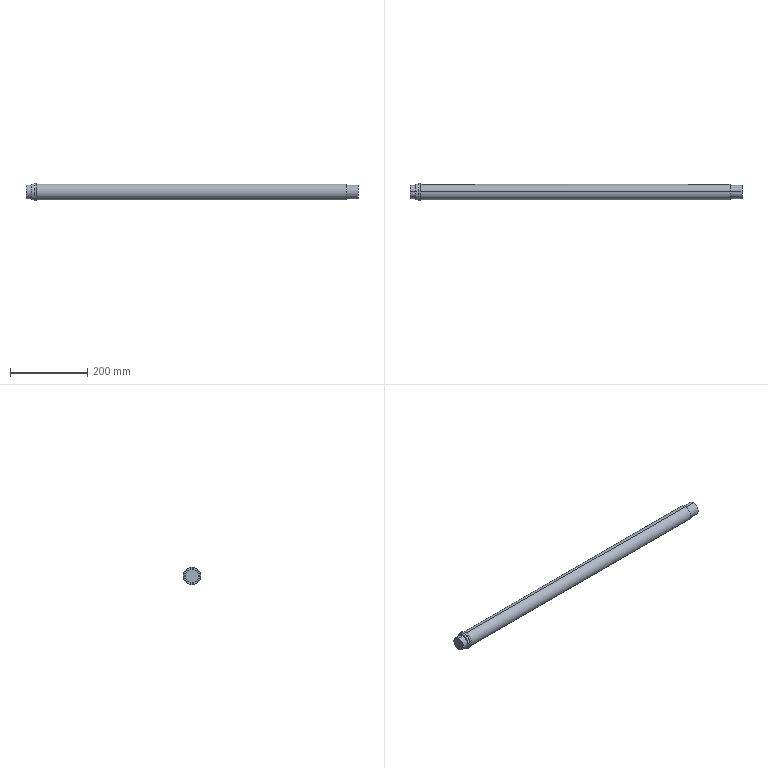Part | SolidWorks | features ICE 5, Extrusion 1 | 1 solid | 26 faces | box 859 x 45 x 45 mm | volume 1051730 mm3 | cylinder 14 | plane 12 | commonest cylinder face diameters 12 x4 35 x4 40 x2 41 x2 45 x2
STEP:
#1=CARTESIAN_POINT('',(-26.,0.,17.5));
#2=VERTEX_POINT('',#1);
#3=CARTESIAN_POINT('',(-26.,0.,-17.5));
#4=VERTEX_POINT('',#3);
#5=CARTESIAN_POINT('',(-26.,0.,0.));
#6=DIRECTION('',(-1.,0.,0.));
#7=DIRECTION('',(0.,0.,1.));
#8=AXIS2_PLACEMENT_3D('',#5,#6,#7);
#9=CIRCLE('',#8,17.5);
#10=EDGE_CURVE('',#2,#4,#9,.T.);
#11=ORIENTED_EDGE('',*,*,#10,.F.);
#12=CARTESIAN_POINT('',(-11.,0.,17.5));
#13=VERTEX_POINT('',#12);
#14=CARTESIAN_POINT('',(-26.,0.,17.5));
#15=DIRECTION('',(1.,0.,0.));
#16=VECTOR('',#15,1000.);
#17=LINE('',#14,#16);
#18=EDGE_CURVE('',#2,#13,#17,.T.);
#19=ORIENTED_EDGE('',*,*,#18,.T.);
#20=CARTESIAN_POINT('',(-11.,0.,-17.5));
#21=VERTEX_POINT('',#20);
#22=CARTESIAN_POINT('',(-11.,0.,0.));
#23=DIRECTION('',(-1.,0.,0.));
#24=DIRECTION('',(0.,0.,1.));
#25=AXIS2_PLACEMENT_3D('',#22,#23,#24);
#26=CIRCLE('',#25,17.5);
#27=EDGE_CURVE('',#13,#21,#26,.T.);
#28=ORIENTED_EDGE('',*,*,#27,.T.);
#29=CARTESIAN_POINT('',(-26.,0.,-17.5));
#30=DIRECTION('',(1.,0.,0.));
#31=VECTOR('',#30,1000.);
#32=LINE('',#29,#31);
#33=EDGE_CURVE('',#4,#21,#32,.T.);
#34=ORIENTED_EDGE('',*,*,#33,.F.);
#35=EDGE_LOOP('',(#11,#19,#28,#34));
#36=FACE_OUTER_BOUND('',#35,.T.);
#37=CARTESIAN_POINT('',(-26.,0.,0.));
#38=DIRECTION('',(1.,0.,0.));
#39=DIRECTION('',(0.,0.,-1.));
#40=AXIS2_PLACEMENT_3D('',#37,#38,#39);
#41=CYLINDRICAL_SURFACE('',#40,17.5);
#42=ADVANCED_FACE('',(#36),#41,.T.);
#43=CARTESIAN_POINT('',(-11.,0.,20.5));
#44=VERTEX_POINT('',#43);
#45=CARTESIAN_POINT('',(-11.,0.,-20.5));
#46=VERTEX_POINT('',#45);
#47=CARTESIAN_POINT('',(-11.,0.,0.));
#48=DIRECTION('',(-1.,0.,0.));
#49=DIRECTION('',(0.,0.,1.));
#50=AXIS2_PLACEMENT_3D('',#47,#48,#49);
#51=CIRCLE('',#50,20.5);
#52=EDGE_CURVE('',#44,#46,#51,.T.);
#53=ORIENTED_EDGE('',*,*,#52,.F.);
#54=CARTESIAN_POINT('',(-5.,0.,20.5));
#55=VERTEX_POINT('',#54);
#56=CARTESIAN_POINT('',(-11.,0.,20.5));
#57=DIRECTION('',(1.,0.,0.));
#58=VECTOR('',#57,1000.);
#59=LINE('',#56,#58);
#60=EDGE_CURVE('',#44,#55,#59,.T.);
#61=ORIENTED_EDGE('',*,*,#60,.T.);
#62=CARTESIAN_POINT('',(-5.,0.,-20.5));
#63=VERTEX_POINT('',#62);
#64=CARTESIAN_POINT('',(-5.,0.,0.));
#65=DIRECTION('',(-1.,0.,0.));
#66=DIRECTION('',(0.,0.,1.));
#67=AXIS2_PLACEMENT_3D('',#64,#65,#66);
#68=CIRCLE('',#67,20.5);
#69=EDGE_CURVE('',#55,#63,#68,.T.);
#70=ORIENTED_EDGE('',*,*,#69,.T.);
#71=CARTESIAN_POINT('',(-11.,0.,-20.5));
#72=DIRECTION('',(1.,0.,0.));
#73=VECTOR('',#72,1000.);
#74=LINE('',#71,#73);
#75=EDGE_CURVE('',#46,#63,#74,.T.);
#76=ORIENTED_EDGE('',*,*,#75,.F.);
#77=EDGE_LOOP('',(#53,#61,#70,#76));
#78=FACE_OUTER_BOUND('',#77,.T.);
#79=CARTESIAN_POINT('',(-11.,0.,0.));
#80=DIRECTION('',(1.,0.,0.));
#81=DIRECTION('',(0.,0.,-1.));
#82=AXIS2_PLACEMENT_3D('',#79,#80,#81);
#83=CYLINDRICAL_SURFACE('',#82,20.5);
#84=ADVANCED_FACE('',(#78),#83,.T.);
#85=CARTESIAN_POINT('',(-5.,0.,22.5));
#86=VERTEX_POINT('',#85);
#87=CARTESIAN_POINT('',(-5.,0.,-22.5));
#88=VERTEX_POINT('',#87);
#89=CARTESIAN_POINT('',(-5.,0.,0.));
#90=DIRECTION('',(-1.,0.,0.));
#91=DIRECTION('',(0.,0.,1.));
#92=AXIS2_PLACEMENT_3D('',#89,#90,#91);
#93=CIRCLE('',#92,22.5);
#94=EDGE_CURVE('',#86,#88,#93,.T.);
#95=ORIENTED_EDGE('',*,*,#94,.F.);
#96=CARTESIAN_POINT('',(0.,0.,22.5));
#97=VERTEX_POINT('',#96);
#98=CARTESIAN_POINT('',(-5.,0.,22.5));
#99=DIRECTION('',(1.,0.,0.));
#100=VECTOR('',#99,1000.);
#101=LINE('',#98,#100);
#102=EDGE_CURVE('',#86,#97,#101,.T.);
#103=ORIENTED_EDGE('',*,*,#102,.T.);
#104=CARTESIAN_POINT('',(0.,0.,-22.5));
#105=VERTEX_POINT('',#104);
#106=CARTESIAN_POINT('',(0.,0.,0.));
#107=DIRECTION('',(-1.,0.,0.));
#108=DIRECTION('',(0.,0.,1.));
#109=AXIS2_PLACEMENT_3D('',#106,#107,#108);
#110=CIRCLE('',#109,22.5);
#111=EDGE_CURVE('',#97,#105,#110,.T.);
#112=ORIENTED_EDGE('',*,*,#111,.T.);
#113=CARTESIAN_POINT('',(-5.,0.,-22.5));
#114=DIRECTION('',(1.,0.,0.));
#115=VECTOR('',#114,1000.);
#116=LINE('',#113,#115);
#117=EDGE_CURVE('',#88,#105,#116,.T.);
#118=ORIENTED_EDGE('',*,*,#117,.F.);
#119=EDGE_LOOP('',(#95,#103,#112,#118));
#120=FACE_OUTER_BOUND('',#119,.T.);
#121=CARTESIAN_POINT('',(-5.,0.,0.));
#122=DIRECTION('',(1.,0.,0.));
#123=DIRECTION('',(0.,0.,-1.));
#124=AXIS2_PLACEMENT_3D('',#121,#122,#123);
#125=CYLINDRICAL_SURFACE('',#124,22.5);
#126=ADVANCED_FACE('',(#120),#125,.T.);
#127=CARTESIAN_POINT('',(833.,0.,-17.5));
#128=VERTEX_POINT('',#127);
#129=CARTESIAN_POINT('',(833.,0.,17.5));
#130=VERTEX_POINT('',#129);
#131=CARTESIAN_POINT('',(833.,0.,0.));
#132=DIRECTION('',(1.,0.,0.));
#133=DIRECTION('',(0.,0.,-1.));
#134=AXIS2_PLACEMENT_3D('',#131,#132,#133);
#135=CIRCLE('',#134,17.5);
#136=EDGE_CURVE('',#128,#130,#135,.T.);
#137=ORIENTED_EDGE('',*,*,#136,.F.);
#138=CARTESIAN_POINT('',(803.,0.,-17.5));
#139=VERTEX_POINT('',#138);
#140=CARTESIAN_POINT('',(833.,0.,-17.5));
#141=DIRECTION('',(-1.,0.,0.));
#142=VECTOR('',#141,1000.);
#143=LINE('',#140,#142);
#144=EDGE_CURVE('',#128,#139,#143,.T.);
#145=ORIENTED_EDGE('',*,*,#144,.T.);
#146=CARTESIAN_POINT('',(803.,0.,17.5));
#147=VERTEX_POINT('',#146);
#148=CARTESIAN_POINT('',(803.,0.,0.));
#149=DIRECTION('',(1.,0.,0.));
#150=DIRECTION('',(0.,0.,-1.));
#151=AXIS2_PLACEMENT_3D('',#148,#149,#150);
#152=CIRCLE('',#151,17.5);
#153=EDGE_CURVE('',#139,#147,#152,.T.);
#154=ORIENTED_EDGE('',*,*,#153,.T.);
#155=CARTESIAN_POINT('',(833.,0.,17.5));
#156=DIRECTION('',(-1.,0.,0.));
#157=VECTOR('',#156,1000.);
#158=LINE('',#155,#157);
#159=EDGE_CURVE('',#130,#147,#158,.T.);
#160=ORIENTED_EDGE('',*,*,#159,.F.);
#161=EDGE_LOOP('',(#137,#145,#154,#160));
#162=FACE_OUTER_BOUND('',#161,.T.);
#163=CARTESIAN_POINT('',(833.,0.,0.));
#164=DIRECTION('',(-1.,0.,0.));
#165=DIRECTION('',(0.,0.,1.));
#166=AXIS2_PLACEMENT_3D('',#163,#164,#165);
#167=CYLINDRICAL_SURFACE('',#166,17.5);
#168=ADVANCED_FACE('',(#162),#167,.T.);
#169=CARTESIAN_POINT('',(794.,19.079,6.));
#170=VERTEX_POINT('',#169);
#171=CARTESIAN_POINT('',(696.,19.079,6.));
#172=VERTEX_POINT('',#171);
#173=CARTESIAN_POINT('',(803.,19.079,6.));
#174=DIRECTION('',(-1.,0.,0.));
#175=VECTOR('',#174,1000.);
#176=LINE('',#173,#175);
#177=EDGE_CURVE('',#170,#172,#176,.T.);
#178=ORIENTED_EDGE('',*,*,#177,.T.);
#179=CARTESIAN_POINT('',(696.,19.079,-6.));
#180=VERTEX_POINT('',#179);
#181=CARTESIAN_POINT('',(696.,19.079,6.));
#182=CARTESIAN_POINT('',(695.601,19.079,6.));
#183=CARTESIAN_POINT('',(695.209,19.091,5.961));
#184=CARTESIAN_POINT('',(694.632,19.127,5.845));
#185=CARTESIAN_POINT('',(694.441,19.141,5.797));
#186=CARTESIAN_POINT('',(694.063,19.176,5.682));
#187=CARTESIAN_POINT('',(693.876,19.196,5.615));
#188=CARTESIAN_POINT('',(693.332,19.261,5.388));
#189=CARTESIAN_POINT('',(692.988,19.312,5.204));
#190=CARTESIAN_POINT('',(692.5,19.396,4.877));
#191=CARTESIAN_POINT('',(692.341,19.426,4.759));
#192=CARTESIAN_POINT('',(692.038,19.485,4.51));
#193=CARTESIAN_POINT('',(691.894,19.515,4.379));
#194=CARTESIAN_POINT('',(691.482,19.605,3.967));
#195=CARTESIAN_POINT('',(691.234,19.664,3.666));
#196=CARTESIAN_POINT('',(690.795,19.775,3.011));
#197=CARTESIAN_POINT('',(690.61,19.825,2.665));
#198=CARTESIAN_POINT('',(690.385,19.888,2.124));
#199=CARTESIAN_POINT('',(690.319,19.907,1.94));
#200=CARTESIAN_POINT('',(690.204,19.94,1.563));
#201=CARTESIAN_POINT('',(690.155,19.954,1.369));
#202=CARTESIAN_POINT('',(690.039,19.988,0.7875));
#203=CARTESIAN_POINT('',(690.,20.,0.3966));
#204=CARTESIAN_POINT('',(690.,20.,-0.3914));
#205=CARTESIAN_POINT('',(690.039,19.988,-0.7916));
#206=CARTESIAN_POINT('',(690.194,19.943,-1.563));
#207=CARTESIAN_POINT('',(690.308,19.909,-1.938));
#208=CARTESIAN_POINT('',(690.611,19.825,-2.668));
#209=CARTESIAN_POINT('',(690.798,19.774,-3.015));
#210=CARTESIAN_POINT('',(691.123,19.692,-3.501));
#211=CARTESIAN_POINT('',(691.24,19.663,-3.657));
#212=CARTESIAN_POINT('',(691.488,19.605,-3.96));
#213=CARTESIAN_POINT('',(691.621,19.574,-4.106));
#214=CARTESIAN_POINT('',(692.037,19.484,-4.522));
#215=CARTESIAN_POINT('',(692.337,19.425,-4.768));
#216=CARTESIAN_POINT('',(692.985,19.313,-5.202));
#217=CARTESIAN_POINT('',(693.337,19.26,-5.391));
#218=CARTESIAN_POINT('',(694.06,19.174,-5.691));
#219=CARTESIAN_POINT('',(694.434,19.139,-5.805));
#220=CARTESIAN_POINT('',(695.015,19.103,-5.922));
#221=CARTESIAN_POINT('',(695.213,19.094,-5.951));
#222=CARTESIAN_POINT('',(695.607,19.082,-5.99));
#223=CARTESIAN_POINT('',(695.803,19.079,-6.));
#224=CARTESIAN_POINT('',(696.,19.079,-6.));
#225=B_SPLINE_CURVE_WITH_KNOTS('',3,(#181,#182,#183,#184,#185,#186,#187,#188,#189,#190,#191,#192,#193,#194,#195,#196,#197,#198,#199,#200,#201,#202,#203,#204,#205,#206,#207,#208,#209,#210,#211,#212,#213,#214,#215,#216,#217,#218,#219,#220,#221,#222,#223,#224),.UNSPECIFIED.,.F.,.F.,(4,2,2,2,2,2,2,2,2,2,2,2,2,2,2,2,2,2,2,2,2,4),(0.,0.001179,0.001769,0.002358,0.003538,0.004127,0.004717,0.005896,0.007075,0.007665,0.008255,0.009434,0.01061,0.01179,0.01297,0.01356,0.01415,0.01533,0.01651,0.01769,0.01828,0.01887),.UNSPECIFIED.);
#226=EDGE_CURVE('',#172,#180,#225,.T.);
#227=ORIENTED_EDGE('',*,*,#226,.T.);
#228=CARTESIAN_POINT('',(794.,19.079,-6.));
#229=VERTEX_POINT('',#228);
#230=CARTESIAN_POINT('',(803.,19.079,-6.));
#231=DIRECTION('',(1.,0.,0.));
#232=VECTOR('',#231,1000.);
#233=LINE('',#230,#232);
#234=EDGE_CURVE('',#180,#229,#233,.T.);
#235=ORIENTED_EDGE('',*,*,#234,.T.);
#236=CARTESIAN_POINT('',(794.,19.079,-6.));
#237=CARTESIAN_POINT('',(794.393,19.079,-6.));
#238=CARTESIAN_POINT('',(794.787,19.091,-5.961));
#239=CARTESIAN_POINT('',(795.566,19.139,-5.806));
#240=CARTESIAN_POINT('',(795.941,19.174,-5.691));
#241=CARTESIAN_POINT('',(796.664,19.261,-5.39));
#242=CARTESIAN_POINT('',(797.015,19.313,-5.202));
#243=CARTESIAN_POINT('',(797.664,19.425,-4.767));
#244=CARTESIAN_POINT('',(797.965,19.484,-4.521));
#245=CARTESIAN_POINT('',(798.38,19.575,-4.105));
#246=CARTESIAN_POINT('',(798.513,19.605,-3.959));
#247=CARTESIAN_POINT('',(798.761,19.664,-3.657));
#248=CARTESIAN_POINT('',(798.877,19.692,-3.5));
#249=CARTESIAN_POINT('',(799.202,19.774,-3.015));
#250=CARTESIAN_POINT('',(799.388,19.824,-2.67));
#251=CARTESIAN_POINT('',(799.692,19.909,-1.939));
#252=CARTESIAN_POINT('',(799.806,19.943,-1.564));
#253=CARTESIAN_POINT('',(799.922,19.977,-0.9868));
#254=CARTESIAN_POINT('',(799.951,19.985,-0.7922));
#255=CARTESIAN_POINT('',(799.99,19.997,-0.398));
#256=CARTESIAN_POINT('',(800.,20.,-0.1981));
#257=CARTESIAN_POINT('',(800.,20.,0.3951));
#258=CARTESIAN_POINT('',(799.961,19.988,0.7861));
#259=CARTESIAN_POINT('',(799.846,19.954,1.366));
#260=CARTESIAN_POINT('',(799.797,19.94,1.559));
#261=CARTESIAN_POINT('',(799.682,19.907,1.938));
#262=CARTESIAN_POINT('',(799.615,19.888,2.123));
#263=CARTESIAN_POINT('',(799.39,19.825,2.665));
#264=CARTESIAN_POINT('',(799.205,19.775,3.01));
#265=CARTESIAN_POINT('',(798.766,19.664,3.666));
#266=CARTESIAN_POINT('',(798.519,19.605,3.967));
#267=CARTESIAN_POINT('',(798.106,19.515,4.379));
#268=CARTESIAN_POINT('',(797.962,19.485,4.51));
#269=CARTESIAN_POINT('',(797.659,19.426,4.759));
#270=CARTESIAN_POINT('',(797.5,19.397,4.877));
#271=CARTESIAN_POINT('',(797.012,19.312,5.204));
#272=CARTESIAN_POINT('',(796.669,19.261,5.388));
#273=CARTESIAN_POINT('',(795.946,19.174,5.689));
#274=CARTESIAN_POINT('',(795.563,19.139,5.806));
#275=CARTESIAN_POINT('',(794.791,19.091,5.961));
#276=CARTESIAN_POINT('',(794.399,19.079,6.));
#277=CARTESIAN_POINT('',(794.,19.079,6.));
#278=B_SPLINE_CURVE_WITH_KNOTS('',3,(#236,#237,#238,#239,#240,#241,#242,#243,#244,#245,#246,#247,#248,#249,#250,#251,#252,#253,#254,#255,#256,#257,#258,#259,#260,#261,#262,#263,#264,#265,#266,#267,#268,#269,#270,#271,#272,#273,#274,#275,#276,#277),.UNSPECIFIED.,.F.,.F.,(4,2,2,2,2,2,2,2,2,2,2,2,2,2,2,2,2,2,2,2,4),(0.01887,0.02005,0.02123,0.0224,0.02358,0.02417,0.02476,0.02594,0.02712,0.02771,0.0283,0.02948,0.03007,0.03066,0.03184,0.03301,0.0336,0.03419,0.03537,0.03655,0.03773),.UNSPECIFIED.);
#279=EDGE_CURVE('',#229,#170,#278,.T.);
#280=ORIENTED_EDGE('',*,*,#279,.T.);
#281=EDGE_LOOP('',(#178,#227,#235,#280));
#282=FACE_BOUND('',#281,.T.);
#283=CARTESIAN_POINT('',(9.,19.079,-6.));
#284=VERTEX_POINT('',#283);
#285=CARTESIAN_POINT('',(137.,19.079,-6.));
#286=VERTEX_POINT('',#285);
#287=CARTESIAN_POINT('',(803.,19.079,-6.));
#288=DIRECTION('',(1.,0.,0.));
#289=VECTOR('',#288,1000.);
#290=LINE('',#287,#289);
#291=EDGE_CURVE('',#284,#286,#290,.T.);
#292=ORIENTED_EDGE('',*,*,#291,.T.);
#293=CARTESIAN_POINT('',(137.,19.079,6.));
#294=VERTEX_POINT('',#293);
#295=CARTESIAN_POINT('',(137.,19.079,-6.));
#296=CARTESIAN_POINT('',(137.393,19.079,-6.));
#297=CARTESIAN_POINT('',(137.787,19.091,-5.961));
#298=CARTESIAN_POINT('',(138.566,19.139,-5.806));
#299=CARTESIAN_POINT('',(138.941,19.174,-5.691));
#300=CARTESIAN_POINT('',(139.664,19.261,-5.39));
#301=CARTESIAN_POINT('',(140.015,19.313,-5.202));
#302=CARTESIAN_POINT('',(140.664,19.425,-4.767));
#303=CARTESIAN_POINT('',(140.965,19.484,-4.521));
#304=CARTESIAN_POINT('',(141.38,19.575,-4.105));
#305=CARTESIAN_POINT('',(141.513,19.605,-3.959));
#306=CARTESIAN_POINT('',(141.761,19.664,-3.657));
#307=CARTESIAN_POINT('',(141.877,19.692,-3.5));
#308=CARTESIAN_POINT('',(142.202,19.774,-3.015));
#309=CARTESIAN_POINT('',(142.388,19.824,-2.67));
#310=CARTESIAN_POINT('',(142.692,19.909,-1.939));
#311=CARTESIAN_POINT('',(142.806,19.943,-1.564));
#312=CARTESIAN_POINT('',(142.922,19.977,-0.9868));
#313=CARTESIAN_POINT('',(142.951,19.985,-0.7922));
#314=CARTESIAN_POINT('',(142.99,19.997,-0.398));
#315=CARTESIAN_POINT('',(143.,20.,-0.1981));
#316=CARTESIAN_POINT('',(143.,20.,0.3951));
#317=CARTESIAN_POINT('',(142.961,19.988,0.7861));
#318=CARTESIAN_POINT('',(142.846,19.954,1.366));
#319=CARTESIAN_POINT('',(142.797,19.94,1.559));
#320=CARTESIAN_POINT('',(142.682,19.907,1.938));
#321=CARTESIAN_POINT('',(142.615,19.888,2.123));
#322=CARTESIAN_POINT('',(142.39,19.825,2.665));
#323=CARTESIAN_POINT('',(142.205,19.775,3.01));
#324=CARTESIAN_POINT('',(141.766,19.664,3.666));
#325=CARTESIAN_POINT('',(141.519,19.605,3.967));
#326=CARTESIAN_POINT('',(141.106,19.515,4.379));
#327=CARTESIAN_POINT('',(140.962,19.485,4.51));
#328=CARTESIAN_POINT('',(140.659,19.426,4.759));
#329=CARTESIAN_POINT('',(140.5,19.397,4.877));
#330=CARTESIAN_POINT('',(140.012,19.312,5.204));
#331=CARTESIAN_POINT('',(139.669,19.261,5.388));
#332=CARTESIAN_POINT('',(138.946,19.174,5.689));
#333=CARTESIAN_POINT('',(138.563,19.139,5.806));
#334=CARTESIAN_POINT('',(137.791,19.091,5.961));
#335=CARTESIAN_POINT('',(137.399,19.079,6.));
#336=CARTESIAN_POINT('',(137.,19.079,6.));
#337=B_SPLINE_CURVE_WITH_KNOTS('',3,(#295,#296,#297,#298,#299,#300,#301,#302,#303,#304,#305,#306,#307,#308,#309,#310,#311,#312,#313,#314,#315,#316,#317,#318,#319,#320,#321,#322,#323,#324,#325,#326,#327,#328,#329,#330,#331,#332,#333,#334,#335,#336),.UNSPECIFIED.,.F.,.F.,(4,2,2,2,2,2,2,2,2,2,2,2,2,2,2,2,2,2,2,2,4),(0.01887,0.02005,0.02123,0.0224,0.02358,0.02417,0.02476,0.02594,0.02712,0.02771,0.0283,0.02948,0.03007,0.03066,0.03184,0.03301,0.0336,0.03419,0.03537,0.03655,0.03773),.UNSPECIFIED.);
#338=EDGE_CURVE('',#286,#294,#337,.T.);
#339=ORIENTED_EDGE('',*,*,#338,.T.);
#340=CARTESIAN_POINT('',(9.,19.079,6.));
#341=VERTEX_POINT('',#340);
#342=CARTESIAN_POINT('',(803.,19.079,6.));
#343=DIRECTION('',(-1.,0.,0.));
#344=VECTOR('',#343,1000.);
#345=LINE('',#342,#344);
#346=EDGE_CURVE('',#294,#341,#345,.T.);
#347=ORIENTED_EDGE('',*,*,#346,.T.);
#348=CARTESIAN_POINT('',(9.,19.079,6.));
#349=CARTESIAN_POINT('',(8.601,19.079,6.));
#350=CARTESIAN_POINT('',(8.209,19.091,5.961));
#351=CARTESIAN_POINT('',(7.632,19.127,5.845));
#352=CARTESIAN_POINT('',(7.441,19.141,5.797));
#353=CARTESIAN_POINT('',(7.063,19.176,5.682));
#354=CARTESIAN_POINT('',(6.876,19.196,5.615));
#355=CARTESIAN_POINT('',(6.332,19.261,5.388));
#356=CARTESIAN_POINT('',(5.988,19.312,5.204));
#357=CARTESIAN_POINT('',(5.5,19.396,4.877));
#358=CARTESIAN_POINT('',(5.341,19.426,4.759));
#359=CARTESIAN_POINT('',(5.038,19.485,4.51));
#360=CARTESIAN_POINT('',(4.894,19.515,4.379));
#361=CARTESIAN_POINT('',(4.482,19.605,3.967));
#362=CARTESIAN_POINT('',(4.234,19.664,3.666));
#363=CARTESIAN_POINT('',(3.795,19.775,3.011));
#364=CARTESIAN_POINT('',(3.61,19.825,2.665));
#365=CARTESIAN_POINT('',(3.385,19.888,2.124));
#366=CARTESIAN_POINT('',(3.319,19.907,1.94));
#367=CARTESIAN_POINT('',(3.204,19.94,1.563));
#368=CARTESIAN_POINT('',(3.155,19.954,1.369));
#369=CARTESIAN_POINT('',(3.039,19.988,0.7875));
#370=CARTESIAN_POINT('',(3.,20.,0.3966));
#371=CARTESIAN_POINT('',(3.,20.,-0.3914));
#372=CARTESIAN_POINT('',(3.039,19.988,-0.7916));
#373=CARTESIAN_POINT('',(3.194,19.943,-1.563));
#374=CARTESIAN_POINT('',(3.308,19.909,-1.938));
#375=CARTESIAN_POINT('',(3.611,19.825,-2.668));
#376=CARTESIAN_POINT('',(3.798,19.774,-3.015));
#377=CARTESIAN_POINT('',(4.123,19.692,-3.501));
#378=CARTESIAN_POINT('',(4.24,19.663,-3.657));
#379=CARTESIAN_POINT('',(4.488,19.605,-3.96));
#380=CARTESIAN_POINT('',(4.621,19.574,-4.106));
#381=CARTESIAN_POINT('',(5.037,19.484,-4.522));
#382=CARTESIAN_POINT('',(5.337,19.425,-4.768));
#383=CARTESIAN_POINT('',(5.985,19.313,-5.202));
#384=CARTESIAN_POINT('',(6.337,19.26,-5.391));
#385=CARTESIAN_POINT('',(7.06,19.174,-5.691));
#386=CARTESIAN_POINT('',(7.434,19.139,-5.805));
#387=CARTESIAN_POINT('',(8.015,19.103,-5.922));
#388=CARTESIAN_POINT('',(8.213,19.094,-5.951));
#389=CARTESIAN_POINT('',(8.607,19.082,-5.99));
#390=CARTESIAN_POINT('',(8.803,19.079,-6.));
#391=CARTESIAN_POINT('',(9.,19.079,-6.));
#392=B_SPLINE_CURVE_WITH_KNOTS('',3,(#348,#349,#350,#351,#352,#353,#354,#355,#356,#357,#358,#359,#360,#361,#362,#363,#364,#365,#366,#367,#368,#369,#370,#371,#372,#373,#374,#375,#376,#377,#378,#379,#380,#381,#382,#383,#384,#385,#386,#387,#388,#389,#390,#391),.UNSPECIFIED.,.F.,.F.,(4,2,2,2,2,2,2,2,2,2,2,2,2,2,2,2,2,2,2,2,2,4),(0.,0.001179,0.001769,0.002358,0.003538,0.004127,0.004717,0.005896,0.007075,0.007665,0.008255,0.009434,0.01061,0.01179,0.01297,0.01356,0.01415,0.01533,0.01651,0.01769,0.01828,0.01887),.UNSPECIFIED.);
#393=EDGE_CURVE('',#341,#284,#392,.T.);
#394=ORIENTED_EDGE('',*,*,#393,.T.);
#395=EDGE_LOOP('',(#292,#339,#347,#394));
#396=FACE_BOUND('',#395,.T.);
#397=CARTESIAN_POINT('',(803.,0.,-20.));
#398=VERTEX_POINT('',#397);
#399=CARTESIAN_POINT('',(803.,0.,20.));
#400=VERTEX_POINT('',#399);
#401=CARTESIAN_POINT('',(803.,0.,0.));
#402=DIRECTION('',(1.,0.,0.));
#403=DIRECTION('',(0.,0.,-1.));
#404=AXIS2_PLACEMENT_3D('',#401,#402,#403);
#405=CIRCLE('',#404,20.);
#406=EDGE_CURVE('',#398,#400,#405,.T.);
#407=ORIENTED_EDGE('',*,*,#406,.F.);
#408=CARTESIAN_POINT('',(0.,0.,-20.));
#409=VERTEX_POINT('',#408);
#410=CARTESIAN_POINT('',(803.,0.,-20.));
#411=DIRECTION('',(-1.,0.,0.));
#412=VECTOR('',#411,1000.);
#413=LINE('',#410,#412);
#414=EDGE_CURVE('',#398,#409,#413,.T.);
#415=ORIENTED_EDGE('',*,*,#414,.T.);
#416=CARTESIAN_POINT('',(0.,0.,20.));
#417=VERTEX_POINT('',#416);
#418=CARTESIAN_POINT('',(0.,0.,0.));
#419=DIRECTION('',(-1.,0.,0.));
#420=DIRECTION('',(0.,0.,1.));
#421=AXIS2_PLACEMENT_3D('',#418,#419,#420);
#422=CIRCLE('',#421,20.);
#423=EDGE_CURVE('',#417,#409,#422,.T.);
#424=ORIENTED_EDGE('',*,*,#423,.F.);
#425=CARTESIAN_POINT('',(803.,0.,20.));
#426=DIRECTION('',(-1.,0.,0.));
#427=VECTOR('',#426,1000.);
#428=LINE('',#425,#427);
#429=EDGE_CURVE('',#400,#417,#428,.T.);
#430=ORIENTED_EDGE('',*,*,#429,.F.);
#431=EDGE_LOOP('',(#407,#415,#424,#430));
#432=FACE_OUTER_BOUND('',#431,.T.);
#433=CARTESIAN_POINT('',(803.,0.,0.));
#434=DIRECTION('',(-1.,0.,0.));
#435=DIRECTION('',(0.,0.,1.));
#436=AXIS2_PLACEMENT_3D('',#433,#434,#435);
#437=CYLINDRICAL_SURFACE('',#436,20.);
#438=ADVANCED_FACE('',(#282,#396,#432),#437,.T.);
#439=CARTESIAN_POINT('',(-11.,0.,0.));
#440=DIRECTION('',(-1.,0.,0.));
#441=DIRECTION('',(0.,0.,1.));
#442=AXIS2_PLACEMENT_3D('',#439,#440,#441);
#443=CIRCLE('',#442,20.5);
#444=EDGE_CURVE('',#46,#44,#443,.T.);
#445=ORIENTED_EDGE('',*,*,#444,.T.);
#446=ORIENTED_EDGE('',*,*,#52,.T.);
#447=EDGE_LOOP('',(#445,#446));
#448=FACE_OUTER_BOUND('',#447,.T.);
#449=CARTESIAN_POINT('',(-11.,0.,0.));
#450=DIRECTION('',(-1.,0.,0.));
#451=DIRECTION('',(0.,0.,1.));
#452=AXIS2_PLACEMENT_3D('',#449,#450,#451);
#453=CIRCLE('',#452,17.5);
#454=EDGE_CURVE('',#21,#13,#453,.T.);
#455=ORIENTED_EDGE('',*,*,#454,.F.);
#456=ORIENTED_EDGE('',*,*,#27,.F.);
#457=EDGE_LOOP('',(#455,#456));
#458=FACE_BOUND('',#457,.T.);
#459=CARTESIAN_POINT('',(-11.,0.,0.));
#460=DIRECTION('',(-1.,0.,0.));
#461=DIRECTION('',(0.,0.,1.));
#462=AXIS2_PLACEMENT_3D('',#459,#460,#461);
#463=PLANE('',#462);
#464=ADVANCED_FACE('',(#448,#458),#463,.T.);
#465=CARTESIAN_POINT('',(-5.,0.,0.));
#466=DIRECTION('',(-1.,0.,0.));
#467=DIRECTION('',(0.,0.,1.));
#468=AXIS2_PLACEMENT_3D('',#465,#466,#467);
#469=CIRCLE('',#468,22.5);
#470=EDGE_CURVE('',#88,#86,#469,.T.);
#471=ORIENTED_EDGE('',*,*,#470,.T.);
#472=ORIENTED_EDGE('',*,*,#94,.T.);
#473=EDGE_LOOP('',(#471,#472));
#474=FACE_OUTER_BOUND('',#473,.T.);
#475=CARTESIAN_POINT('',(-5.,0.,0.));
#476=DIRECTION('',(-1.,0.,0.));
#477=DIRECTION('',(0.,0.,1.));
#478=AXIS2_PLACEMENT_3D('',#475,#476,#477);
#479=CIRCLE('',#478,20.5);
#480=EDGE_CURVE('',#63,#55,#479,.T.);
#481=ORIENTED_EDGE('',*,*,#480,.F.);
#482=ORIENTED_EDGE('',*,*,#69,.F.);
#483=EDGE_LOOP('',(#481,#482));
#484=FACE_BOUND('',#483,.T.);
#485=CARTESIAN_POINT('',(-5.,0.,0.));
#486=DIRECTION('',(-1.,0.,0.));
#487=DIRECTION('',(0.,0.,1.));
#488=AXIS2_PLACEMENT_3D('',#485,#486,#487);
#489=PLANE('',#488);
#490=ADVANCED_FACE('',(#474,#484),#489,.T.);
#491=CARTESIAN_POINT('',(803.,0.,0.));
#492=DIRECTION('',(1.,0.,0.));
#493=DIRECTION('',(0.,0.,-1.));
#494=AXIS2_PLACEMENT_3D('',#491,#492,#493);
#495=CIRCLE('',#494,20.);
#496=EDGE_CURVE('',#400,#398,#495,.T.);
#497=ORIENTED_EDGE('',*,*,#496,.T.);
#498=ORIENTED_EDGE('',*,*,#406,.T.);
#499=EDGE_LOOP('',(#497,#498));
#500=FACE_OUTER_BOUND('',#499,.T.);
#501=CARTESIAN_POINT('',(803.,0.,0.));
#502=DIRECTION('',(1.,0.,0.));
#503=DIRECTION('',(0.,0.,-1.));
#504=AXIS2_PLACEMENT_3D('',#501,#502,#503);
#505=CIRCLE('',#504,17.5);
#506=EDGE_CURVE('',#147,#139,#505,.T.);
#507=ORIENTED_EDGE('',*,*,#506,.F.);
#508=ORIENTED_EDGE('',*,*,#153,.F.);
#509=EDGE_LOOP('',(#507,#508));
#510=FACE_BOUND('',#509,.T.);
#511=CARTESIAN_POINT('',(803.,0.,0.));
#512=DIRECTION('',(1.,0.,0.));
#513=DIRECTION('',(0.,0.,-1.));
#514=AXIS2_PLACEMENT_3D('',#511,#512,#513);
#515=PLANE('',#514);
#516=ADVANCED_FACE('',(#500,#510),#515,.T.);
#517=ORIENTED_EDGE('',*,*,#414,.F.);
#518=ORIENTED_EDGE('',*,*,#496,.F.);
#519=ORIENTED_EDGE('',*,*,#429,.T.);
#520=CARTESIAN_POINT('',(0.,0.,0.));
#521=DIRECTION('',(-1.,0.,0.));
#522=DIRECTION('',(0.,0.,1.));
#523=AXIS2_PLACEMENT_3D('',#520,#521,#522);
#524=CIRCLE('',#523,20.);
#525=EDGE_CURVE('',#409,#417,#524,.T.);
#526=ORIENTED_EDGE('',*,*,#525,.F.);
#527=EDGE_LOOP('',(#517,#518,#519,#526));
#528=FACE_OUTER_BOUND('',#527,.T.);
#529=CARTESIAN_POINT('',(803.,0.,0.));
#530=DIRECTION('',(-1.,0.,0.));
#531=DIRECTION('',(0.,0.,1.));
#532=AXIS2_PLACEMENT_3D('',#529,#530,#531);
#533=CYLINDRICAL_SURFACE('',#532,20.);
#534=ADVANCED_FACE('',(#528),#533,.T.);
#535=ORIENTED_EDGE('',*,*,#144,.F.);
#536=CARTESIAN_POINT('',(833.,0.,0.));
#537=DIRECTION('',(1.,0.,0.));
#538=DIRECTION('',(0.,0.,-1.));
#539=AXIS2_PLACEMENT_3D('',#536,#537,#538);
#540=CIRCLE('',#539,17.5);
#541=EDGE_CURVE('',#130,#128,#540,.T.);
#542=ORIENTED_EDGE('',*,*,#541,.F.);
#543=ORIENTED_EDGE('',*,*,#159,.T.);
#544=ORIENTED_EDGE('',*,*,#506,.T.);
#545=EDGE_LOOP('',(#535,#542,#543,#544));
#546=FACE_OUTER_BOUND('',#545,.T.);
#547=CARTESIAN_POINT('',(833.,0.,0.));
#548=DIRECTION('',(-1.,0.,0.));
#549=DIRECTION('',(0.,0.,1.));
#550=AXIS2_PLACEMENT_3D('',#547,#548,#549);
#551=CYLINDRICAL_SURFACE('',#550,17.5);
#552=ADVANCED_FACE('',(#546),#551,.T.);
#553=ORIENTED_EDGE('',*,*,#541,.T.);
#554=ORIENTED_EDGE('',*,*,#136,.T.);
#555=EDGE_LOOP('',(#553,#554));
#556=FACE_OUTER_BOUND('',#555,.T.);
#557=CARTESIAN_POINT('',(833.,0.,0.));
#558=DIRECTION('',(1.,0.,0.));
#559=DIRECTION('',(0.,0.,-1.));
#560=AXIS2_PLACEMENT_3D('',#557,#558,#559);
#561=PLANE('',#560);
#562=ADVANCED_FACE('',(#556),#561,.T.);
#563=CARTESIAN_POINT('',(0.,0.,0.));
#564=DIRECTION('',(-1.,0.,0.));
#565=DIRECTION('',(0.,0.,1.));
#566=AXIS2_PLACEMENT_3D('',#563,#564,#565);
#567=CIRCLE('',#566,22.5);
#568=EDGE_CURVE('',#105,#97,#567,.T.);
#569=ORIENTED_EDGE('',*,*,#568,.F.);
#570=ORIENTED_EDGE('',*,*,#111,.F.);
#571=EDGE_LOOP('',(#569,#570));
#572=FACE_OUTER_BOUND('',#571,.T.);
#573=ORIENTED_EDGE('',*,*,#423,.T.);
#574=ORIENTED_EDGE('',*,*,#525,.T.);
#575=EDGE_LOOP('',(#573,#574));
#576=FACE_BOUND('',#575,.T.);
#577=CARTESIAN_POINT('',(0.,0.,0.));
#578=DIRECTION('',(-1.,0.,0.));
#579=DIRECTION('',(0.,0.,1.));
#580=AXIS2_PLACEMENT_3D('',#577,#578,#579);
#581=PLANE('',#580);
#582=ADVANCED_FACE('',(#572,#576),#581,.F.);
#583=ORIENTED_EDGE('',*,*,#102,.F.);
#584=ORIENTED_EDGE('',*,*,#470,.F.);
#585=ORIENTED_EDGE('',*,*,#117,.T.);
#586=ORIENTED_EDGE('',*,*,#568,.T.);
#587=EDGE_LOOP('',(#583,#584,#585,#586));
#588=FACE_OUTER_BOUND('',#587,.T.);
#589=CARTESIAN_POINT('',(-5.,0.,0.));
#590=DIRECTION('',(1.,0.,0.));
#591=DIRECTION('',(0.,0.,-1.));
#592=AXIS2_PLACEMENT_3D('',#589,#590,#591);
#593=CYLINDRICAL_SURFACE('',#592,22.5);
#594=ADVANCED_FACE('',(#588),#593,.T.);
#595=ORIENTED_EDGE('',*,*,#60,.F.);
#596=ORIENTED_EDGE('',*,*,#444,.F.);
#597=ORIENTED_EDGE('',*,*,#75,.T.);
#598=ORIENTED_EDGE('',*,*,#480,.T.);
#599=EDGE_LOOP('',(#595,#596,#597,#598));
#600=FACE_OUTER_BOUND('',#599,.T.);
#601=CARTESIAN_POINT('',(-11.,0.,0.));
#602=DIRECTION('',(1.,0.,0.));
#603=DIRECTION('',(0.,0.,-1.));
#604=AXIS2_PLACEMENT_3D('',#601,#602,#603);
#605=CYLINDRICAL_SURFACE('',#604,20.5);
#606=ADVANCED_FACE('',(#600),#605,.T.);
#607=ORIENTED_EDGE('',*,*,#18,.F.);
#608=CARTESIAN_POINT('',(-26.,0.,0.));
#609=DIRECTION('',(-1.,0.,0.));
#610=DIRECTION('',(0.,0.,1.));
#611=AXIS2_PLACEMENT_3D('',#608,#609,#610);
#612=CIRCLE('',#611,17.5);
#613=EDGE_CURVE('',#4,#2,#612,.T.);
#614=ORIENTED_EDGE('',*,*,#613,.F.);
#615=ORIENTED_EDGE('',*,*,#33,.T.);
#616=ORIENTED_EDGE('',*,*,#454,.T.);
#617=EDGE_LOOP('',(#607,#614,#615,#616));
#618=FACE_OUTER_BOUND('',#617,.T.);
#619=CARTESIAN_POINT('',(-26.,0.,0.));
#620=DIRECTION('',(1.,0.,0.));
#621=DIRECTION('',(0.,0.,-1.));
#622=AXIS2_PLACEMENT_3D('',#619,#620,#621);
#623=CYLINDRICAL_SURFACE('',#622,17.5);
#624=ADVANCED_FACE('',(#618),#623,.T.);
#625=ORIENTED_EDGE('',*,*,#613,.T.);
#626=ORIENTED_EDGE('',*,*,#10,.T.);
#627=EDGE_LOOP('',(#625,#626));
#628=FACE_OUTER_BOUND('',#627,.T.);
#629=CARTESIAN_POINT('',(-26.,0.,0.));
#630=DIRECTION('',(-1.,0.,0.));
#631=DIRECTION('',(0.,0.,1.));
#632=AXIS2_PLACEMENT_3D('',#629,#630,#631);
#633=PLANE('',#632);
#634=ADVANCED_FACE('',(#628),#633,.T.);
#635=CARTESIAN_POINT('',(9.,14.08,6.));
#636=VERTEX_POINT('',#635);
#637=CARTESIAN_POINT('',(9.,14.08,6.));
#638=DIRECTION('',(0.,1.,0.));
#639=VECTOR('',#638,1000.);
#640=LINE('',#637,#639);
#641=EDGE_CURVE('',#636,#341,#640,.T.);
#642=ORIENTED_EDGE('',*,*,#641,.F.);
#643=CARTESIAN_POINT('',(9.,14.08,-6.));
#644=VERTEX_POINT('',#643);
#645=CARTESIAN_POINT('',(9.,14.08,0.));
#646=DIRECTION('',(0.,1.,0.));
#647=DIRECTION('',(0.,0.,1.));
#648=AXIS2_PLACEMENT_3D('',#645,#646,#647);
#649=CIRCLE('',#648,6.);
#650=EDGE_CURVE('',#644,#636,#649,.T.);
#651=ORIENTED_EDGE('',*,*,#650,.F.);
#652=CARTESIAN_POINT('',(9.,14.08,-6.));
#653=DIRECTION('',(0.,1.,0.));
#654=VECTOR('',#653,1000.);
#655=LINE('',#652,#654);
#656=EDGE_CURVE('',#644,#284,#655,.T.);
#657=ORIENTED_EDGE('',*,*,#656,.T.);
#658=ORIENTED_EDGE('',*,*,#393,.F.);
#659=EDGE_LOOP('',(#642,#651,#657,#658));
#660=FACE_OUTER_BOUND('',#659,.T.);
#661=CARTESIAN_POINT('',(9.,14.08,0.));
#662=DIRECTION('',(0.,1.,0.));
#663=DIRECTION('',(0.,0.,1.));
#664=AXIS2_PLACEMENT_3D('',#661,#662,#663);
#665=CYLINDRICAL_SURFACE('',#664,6.);
#666=ADVANCED_FACE('',(#660),#665,.F.);
#667=ORIENTED_EDGE('',*,*,#656,.F.);
#668=CARTESIAN_POINT('',(137.,14.08,-6.));
#669=VERTEX_POINT('',#668);
#670=CARTESIAN_POINT('',(9.,14.08,-6.));
#671=DIRECTION('',(-1.,0.,0.));
#672=VECTOR('',#671,1000.);
#673=LINE('',#670,#672);
#674=EDGE_CURVE('',#669,#644,#673,.T.);
#675=ORIENTED_EDGE('',*,*,#674,.F.);
#676=CARTESIAN_POINT('',(137.,14.08,-6.));
#677=DIRECTION('',(0.,1.,0.));
#678=VECTOR('',#677,1000.);
#679=LINE('',#676,#678);
#680=EDGE_CURVE('',#669,#286,#679,.T.);
#681=ORIENTED_EDGE('',*,*,#680,.T.);
#682=ORIENTED_EDGE('',*,*,#291,.F.);
#683=EDGE_LOOP('',(#667,#675,#681,#682));
#684=FACE_OUTER_BOUND('',#683,.T.);
#685=CARTESIAN_POINT('',(9.,14.08,-6.));
#686=DIRECTION('',(0.,0.,-1.));
#687=DIRECTION('',(-1.,0.,0.));
#688=AXIS2_PLACEMENT_3D('',#685,#686,#687);
#689=PLANE('',#688);
#690=ADVANCED_FACE('',(#684),#689,.F.);
#691=ORIENTED_EDGE('',*,*,#680,.F.);
#692=CARTESIAN_POINT('',(137.,14.08,6.));
#693=VERTEX_POINT('',#692);
#694=CARTESIAN_POINT('',(137.,14.08,0.));
#695=DIRECTION('',(0.,1.,0.));
#696=DIRECTION('',(0.,0.,1.));
#697=AXIS2_PLACEMENT_3D('',#694,#695,#696);
#698=CIRCLE('',#697,6.);
#699=EDGE_CURVE('',#693,#669,#698,.T.);
#700=ORIENTED_EDGE('',*,*,#699,.F.);
#701=CARTESIAN_POINT('',(137.,14.08,6.));
#702=DIRECTION('',(0.,1.,0.));
#703=VECTOR('',#702,1000.);
#704=LINE('',#701,#703);
#705=EDGE_CURVE('',#693,#294,#704,.T.);
#706=ORIENTED_EDGE('',*,*,#705,.T.);
#707=ORIENTED_EDGE('',*,*,#338,.F.);
#708=EDGE_LOOP('',(#691,#700,#706,#707));
#709=FACE_OUTER_BOUND('',#708,.T.);
#710=CARTESIAN_POINT('',(137.,14.08,0.));
#711=DIRECTION('',(0.,1.,0.));
#712=DIRECTION('',(0.,0.,1.));
#713=AXIS2_PLACEMENT_3D('',#710,#711,#712);
#714=CYLINDRICAL_SURFACE('',#713,6.);
#715=ADVANCED_FACE('',(#709),#714,.F.);
#716=ORIENTED_EDGE('',*,*,#705,.F.);
#717=CARTESIAN_POINT('',(9.,14.08,6.));
#718=DIRECTION('',(1.,0.,0.));
#719=VECTOR('',#718,1000.);
#720=LINE('',#717,#719);
#721=EDGE_CURVE('',#636,#693,#720,.T.);
#722=ORIENTED_EDGE('',*,*,#721,.F.);
#723=ORIENTED_EDGE('',*,*,#641,.T.);
#724=ORIENTED_EDGE('',*,*,#346,.F.);
#725=EDGE_LOOP('',(#716,#722,#723,#724));
#726=FACE_OUTER_BOUND('',#725,.T.);
#727=CARTESIAN_POINT('',(9.,14.08,6.));
#728=DIRECTION('',(0.,0.,1.));
#729=DIRECTION('',(1.,0.,0.));
#730=AXIS2_PLACEMENT_3D('',#727,#728,#729);
#731=PLANE('',#730);
#732=ADVANCED_FACE('',(#726),#731,.F.);
#733=ORIENTED_EDGE('',*,*,#650,.T.);
#734=ORIENTED_EDGE('',*,*,#721,.T.);
#735=ORIENTED_EDGE('',*,*,#699,.T.);
#736=ORIENTED_EDGE('',*,*,#674,.T.);
#737=EDGE_LOOP('',(#733,#734,#735,#736));
#738=FACE_OUTER_BOUND('',#737,.T.);
#739=CARTESIAN_POINT('',(9.,14.08,0.));
#740=DIRECTION('',(0.,1.,0.));
#741=DIRECTION('',(0.,0.,1.));
#742=AXIS2_PLACEMENT_3D('',#739,#740,#741);
#743=PLANE('',#742);
#744=ADVANCED_FACE('',(#738),#743,.T.);
#745=CARTESIAN_POINT('',(794.,14.08,-6.));
#746=VERTEX_POINT('',#745);
#747=CARTESIAN_POINT('',(794.,14.08,-6.));
#748=DIRECTION('',(0.,1.,0.));
#749=VECTOR('',#748,1000.);
#750=LINE('',#747,#749);
#751=EDGE_CURVE('',#746,#229,#750,.T.);
#752=ORIENTED_EDGE('',*,*,#751,.F.);
#753=CARTESIAN_POINT('',(794.,14.08,6.));
#754=VERTEX_POINT('',#753);
#755=CARTESIAN_POINT('',(794.,14.08,0.));
#756=DIRECTION('',(0.,1.,0.));
#757=DIRECTION('',(0.,0.,1.));
#758=AXIS2_PLACEMENT_3D('',#755,#756,#757);
#759=CIRCLE('',#758,6.);
#760=EDGE_CURVE('',#754,#746,#759,.T.);
#761=ORIENTED_EDGE('',*,*,#760,.F.);
#762=CARTESIAN_POINT('',(794.,14.08,6.));
#763=DIRECTION('',(0.,1.,0.));
#764=VECTOR('',#763,1000.);
#765=LINE('',#762,#764);
#766=EDGE_CURVE('',#754,#170,#765,.T.);
#767=ORIENTED_EDGE('',*,*,#766,.T.);
#768=ORIENTED_EDGE('',*,*,#279,.F.);
#769=EDGE_LOOP('',(#752,#761,#767,#768));
#770=FACE_OUTER_BOUND('',#769,.T.);
#771=CARTESIAN_POINT('',(794.,14.08,0.));
#772=DIRECTION('',(0.,1.,0.));
#773=DIRECTION('',(0.,0.,1.));
#774=AXIS2_PLACEMENT_3D('',#771,#772,#773);
#775=CYLINDRICAL_SURFACE('',#774,6.);
#776=ADVANCED_FACE('',(#770),#775,.F.);
#777=ORIENTED_EDGE('',*,*,#766,.F.);
#778=CARTESIAN_POINT('',(696.,14.08,6.));
#779=VERTEX_POINT('',#778);
#780=CARTESIAN_POINT('',(794.,14.08,6.));
#781=DIRECTION('',(1.,0.,0.));
#782=VECTOR('',#781,1000.);
#783=LINE('',#780,#782);
#784=EDGE_CURVE('',#779,#754,#783,.T.);
#785=ORIENTED_EDGE('',*,*,#784,.F.);
#786=CARTESIAN_POINT('',(696.,14.08,6.));
#787=DIRECTION('',(0.,1.,0.));
#788=VECTOR('',#787,1000.);
#789=LINE('',#786,#788);
#790=EDGE_CURVE('',#779,#172,#789,.T.);
#791=ORIENTED_EDGE('',*,*,#790,.T.);
#792=ORIENTED_EDGE('',*,*,#177,.F.);
#793=EDGE_LOOP('',(#777,#785,#791,#792));
#794=FACE_OUTER_BOUND('',#793,.T.);
#795=CARTESIAN_POINT('',(794.,14.08,6.));
#796=DIRECTION('',(0.,0.,1.));
#797=DIRECTION('',(1.,0.,0.));
#798=AXIS2_PLACEMENT_3D('',#795,#796,#797);
#799=PLANE('',#798);
#800=ADVANCED_FACE('',(#794),#799,.F.);
#801=ORIENTED_EDGE('',*,*,#790,.F.);
#802=CARTESIAN_POINT('',(696.,14.08,-6.));
#803=VERTEX_POINT('',#802);
#804=CARTESIAN_POINT('',(696.,14.08,0.));
#805=DIRECTION('',(0.,1.,0.));
#806=DIRECTION('',(0.,0.,1.));
#807=AXIS2_PLACEMENT_3D('',#804,#805,#806);
#808=CIRCLE('',#807,6.);
#809=EDGE_CURVE('',#803,#779,#808,.T.);
#810=ORIENTED_EDGE('',*,*,#809,.F.);
#811=CARTESIAN_POINT('',(696.,14.08,-6.));
#812=DIRECTION('',(0.,1.,0.));
#813=VECTOR('',#812,1000.);
#814=LINE('',#811,#813);
#815=EDGE_CURVE('',#803,#180,#814,.T.);
#816=ORIENTED_EDGE('',*,*,#815,.T.);
#817=ORIENTED_EDGE('',*,*,#226,.F.);
#818=EDGE_LOOP('',(#801,#810,#816,#817));
#819=FACE_OUTER_BOUND('',#818,.T.);
#820=CARTESIAN_POINT('',(696.,14.08,0.));
#821=DIRECTION('',(0.,1.,0.));
#822=DIRECTION('',(0.,0.,1.));
#823=AXIS2_PLACEMENT_3D('',#820,#821,#822);
#824=CYLINDRICAL_SURFACE('',#823,6.);
#825=ADVANCED_FACE('',(#819),#824,.F.);
#826=ORIENTED_EDGE('',*,*,#815,.F.);
#827=CARTESIAN_POINT('',(794.,14.08,-6.));
#828=DIRECTION('',(-1.,0.,0.));
#829=VECTOR('',#828,1000.);
#830=LINE('',#827,#829);
#831=EDGE_CURVE('',#746,#803,#830,.T.);
#832=ORIENTED_EDGE('',*,*,#831,.F.);
#833=ORIENTED_EDGE('',*,*,#751,.T.);
#834=ORIENTED_EDGE('',*,*,#234,.F.);
#835=EDGE_LOOP('',(#826,#832,#833,#834));
#836=FACE_OUTER_BOUND('',#835,.T.);
#837=CARTESIAN_POINT('',(794.,14.08,-6.));
#838=DIRECTION('',(0.,0.,-1.));
#839=DIRECTION('',(-1.,0.,0.));
#840=AXIS2_PLACEMENT_3D('',#837,#838,#839);
#841=PLANE('',#840);
#842=ADVANCED_FACE('',(#836),#841,.F.);
#843=ORIENTED_EDGE('',*,*,#760,.T.);
#844=ORIENTED_EDGE('',*,*,#831,.T.);
#845=ORIENTED_EDGE('',*,*,#809,.T.);
#846=ORIENTED_EDGE('',*,*,#784,.T.);
#847=EDGE_LOOP('',(#843,#844,#845,#846));
#848=FACE_OUTER_BOUND('',#847,.T.);
#849=CARTESIAN_POINT('',(794.,14.08,0.));
#850=DIRECTION('',(0.,1.,0.));
#851=DIRECTION('',(0.,0.,1.));
#852=AXIS2_PLACEMENT_3D('',#849,#850,#851);
#853=PLANE('',#852);
#854=ADVANCED_FACE('',(#848),#853,.T.);
#855=CLOSED_SHELL('',(#42,#84,#126,#168,#438,#464,#490,#516,#534,#552,#562,#582,#594,#606,#624,#634,#666,#690,#715,#732,#744,#776,#800,#825,#842,#854));
#856=MANIFOLD_SOLID_BREP('',#855);
#857=CARTESIAN_POINT('',(0.,0.,0.));
#858=DIRECTION('',(0.,0.,1.));
#859=DIRECTION('',(1.,0.,0.));
#860=AXIS2_PLACEMENT_3D('',#857,#858,#859);
#861=(LENGTH_UNIT()NAMED_UNIT(*)SI_UNIT(.MILLI.,.METRE.));
#862=UNCERTAINTY_MEASURE_WITH_UNIT(LENGTH_MEASURE(0.00001),#861,'','');
#863=(NAMED_UNIT(*)PLANE_ANGLE_UNIT()SI_UNIT($,.RADIAN.));
#864=(NAMED_UNIT(*)SI_UNIT($,.STERADIAN.)SOLID_ANGLE_UNIT());
#865=(GEOMETRIC_REPRESENTATION_CONTEXT(3)GLOBAL_UNCERTAINTY_ASSIGNED_CONTEXT((#862))GLOBAL_UNIT_ASSIGNED_CONTEXT((#861,#863,#864))REPRESENTATION_CONTEXT('',''));
#866=ADVANCED_BREP_SHAPE_REPRESENTATION('',(#856,#860),#865);